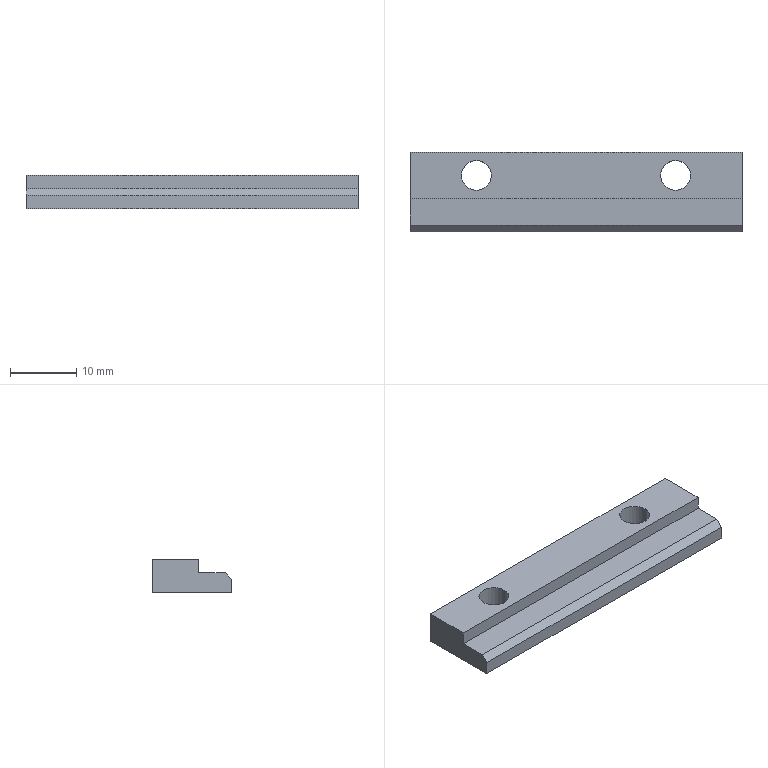Part | SolidWorks | features BaseBody 1 | 1 solid | 13 faces | box 50 x 12 x 5 mm | volume 2316 mm3 | plane 9 | cylinder 4 | commonest cylinder face diameters 4.5 x4
STEP:
#1=CARTESIAN_POINT('',(0.,0.,2.));
#2=VERTEX_POINT('',#1);
#3=CARTESIAN_POINT('',(0.,1.,3.));
#4=VERTEX_POINT('',#3);
#5=CARTESIAN_POINT('',(0.,1.,3.));
#6=DIRECTION('',(0.,0.7071,0.7071));
#7=VECTOR('',#6,1000.);
#8=LINE('',#5,#7);
#9=EDGE_CURVE('',#2,#4,#8,.T.);
#10=ORIENTED_EDGE('',*,*,#9,.F.);
#11=CARTESIAN_POINT('',(50.,0.,2.));
#12=VERTEX_POINT('',#11);
#13=CARTESIAN_POINT('',(0.,0.,2.));
#14=DIRECTION('',(-1.,0.,0.));
#15=VECTOR('',#14,1000.);
#16=LINE('',#13,#15);
#17=EDGE_CURVE('',#12,#2,#16,.T.);
#18=ORIENTED_EDGE('',*,*,#17,.F.);
#19=CARTESIAN_POINT('',(50.,1.,3.));
#20=VERTEX_POINT('',#19);
#21=CARTESIAN_POINT('',(50.,1.,3.));
#22=DIRECTION('',(0.,-0.7071,-0.7071));
#23=VECTOR('',#22,1000.);
#24=LINE('',#21,#23);
#25=EDGE_CURVE('',#20,#12,#24,.T.);
#26=ORIENTED_EDGE('',*,*,#25,.F.);
#27=CARTESIAN_POINT('',(0.,1.,3.));
#28=DIRECTION('',(1.,0.,0.));
#29=VECTOR('',#28,1000.);
#30=LINE('',#27,#29);
#31=EDGE_CURVE('',#4,#20,#30,.T.);
#32=ORIENTED_EDGE('',*,*,#31,.F.);
#33=EDGE_LOOP('',(#10,#18,#26,#32));
#34=FACE_OUTER_BOUND('',#33,.T.);
#35=CARTESIAN_POINT('',(0.,1.,3.));
#36=DIRECTION('',(0.,0.7071,-0.7071));
#37=DIRECTION('',(-1.,0.,0.));
#38=AXIS2_PLACEMENT_3D('',#35,#36,#37);
#39=PLANE('',#38);
#40=ADVANCED_FACE('',(#34),#39,.F.);
#41=CARTESIAN_POINT('',(0.,5.,3.));
#42=VERTEX_POINT('',#41);
#43=CARTESIAN_POINT('',(0.,0.,3.));
#44=DIRECTION('',(0.,1.,0.));
#45=VECTOR('',#44,1000.);
#46=LINE('',#43,#45);
#47=EDGE_CURVE('',#4,#42,#46,.T.);
#48=ORIENTED_EDGE('',*,*,#47,.F.);
#49=ORIENTED_EDGE('',*,*,#31,.T.);
#50=CARTESIAN_POINT('',(50.,5.,3.));
#51=VERTEX_POINT('',#50);
#52=CARTESIAN_POINT('',(50.,0.,3.));
#53=DIRECTION('',(0.,1.,0.));
#54=VECTOR('',#53,1000.);
#55=LINE('',#52,#54);
#56=EDGE_CURVE('',#20,#51,#55,.T.);
#57=ORIENTED_EDGE('',*,*,#56,.T.);
#58=CARTESIAN_POINT('',(0.,5.,3.));
#59=DIRECTION('',(1.,0.,0.));
#60=VECTOR('',#59,1000.);
#61=LINE('',#58,#60);
#62=EDGE_CURVE('',#42,#51,#61,.T.);
#63=ORIENTED_EDGE('',*,*,#62,.F.);
#64=EDGE_LOOP('',(#48,#49,#57,#63));
#65=FACE_OUTER_BOUND('',#64,.T.);
#66=CARTESIAN_POINT('',(0.,0.,3.));
#67=DIRECTION('',(0.,0.,-1.));
#68=DIRECTION('',(0.,-1.,0.));
#69=AXIS2_PLACEMENT_3D('',#66,#67,#68);
#70=PLANE('',#69);
#71=ADVANCED_FACE('',(#65),#70,.F.);
#72=CARTESIAN_POINT('',(50.,5.,5.));
#73=VERTEX_POINT('',#72);
#74=CARTESIAN_POINT('',(50.,5.,5.));
#75=DIRECTION('',(0.,0.,1.));
#76=VECTOR('',#75,1000.);
#77=LINE('',#74,#76);
#78=EDGE_CURVE('',#51,#73,#77,.T.);
#79=ORIENTED_EDGE('',*,*,#78,.T.);
#80=CARTESIAN_POINT('',(0.,5.,5.));
#81=VERTEX_POINT('',#80);
#82=CARTESIAN_POINT('',(0.,5.,5.));
#83=DIRECTION('',(1.,0.,0.));
#84=VECTOR('',#83,1000.);
#85=LINE('',#82,#84);
#86=EDGE_CURVE('',#81,#73,#85,.T.);
#87=ORIENTED_EDGE('',*,*,#86,.F.);
#88=CARTESIAN_POINT('',(0.,5.,5.));
#89=DIRECTION('',(0.,0.,1.));
#90=VECTOR('',#89,1000.);
#91=LINE('',#88,#90);
#92=EDGE_CURVE('',#42,#81,#91,.T.);
#93=ORIENTED_EDGE('',*,*,#92,.F.);
#94=ORIENTED_EDGE('',*,*,#62,.T.);
#95=EDGE_LOOP('',(#79,#87,#93,#94));
#96=FACE_OUTER_BOUND('',#95,.T.);
#97=CARTESIAN_POINT('',(0.,5.,5.));
#98=DIRECTION('',(0.,1.,0.));
#99=DIRECTION('',(1.,0.,0.));
#100=AXIS2_PLACEMENT_3D('',#97,#98,#99);
#101=PLANE('',#100);
#102=ADVANCED_FACE('',(#96),#101,.F.);
#103=CARTESIAN_POINT('',(7.75,8.5,0.));
#104=VERTEX_POINT('',#103);
#105=CARTESIAN_POINT('',(7.75,8.5,5.));
#106=VERTEX_POINT('',#105);
#107=CARTESIAN_POINT('',(7.75,8.5,0.));
#108=DIRECTION('',(0.,0.,1.));
#109=VECTOR('',#108,1000.);
#110=LINE('',#107,#109);
#111=EDGE_CURVE('',#104,#106,#110,.T.);
#112=ORIENTED_EDGE('',*,*,#111,.F.);
#113=CARTESIAN_POINT('',(12.25,8.5,0.));
#114=VERTEX_POINT('',#113);
#115=CARTESIAN_POINT('',(10.,8.5,0.));
#116=DIRECTION('',(0.,0.,1.));
#117=DIRECTION('',(1.,0.,0.));
#118=AXIS2_PLACEMENT_3D('',#115,#116,#117);
#119=CIRCLE('',#118,2.25);
#120=EDGE_CURVE('',#114,#104,#119,.T.);
#121=ORIENTED_EDGE('',*,*,#120,.F.);
#122=CARTESIAN_POINT('',(12.25,8.5,5.));
#123=VERTEX_POINT('',#122);
#124=CARTESIAN_POINT('',(12.25,8.5,0.));
#125=DIRECTION('',(0.,0.,1.));
#126=VECTOR('',#125,1000.);
#127=LINE('',#124,#126);
#128=EDGE_CURVE('',#114,#123,#127,.T.);
#129=ORIENTED_EDGE('',*,*,#128,.T.);
#130=CARTESIAN_POINT('',(10.,8.5,5.));
#131=DIRECTION('',(0.,0.,1.));
#132=DIRECTION('',(1.,0.,0.));
#133=AXIS2_PLACEMENT_3D('',#130,#131,#132);
#134=CIRCLE('',#133,2.25);
#135=EDGE_CURVE('',#123,#106,#134,.T.);
#136=ORIENTED_EDGE('',*,*,#135,.T.);
#137=EDGE_LOOP('',(#112,#121,#129,#136));
#138=FACE_OUTER_BOUND('',#137,.T.);
#139=CARTESIAN_POINT('',(10.,8.5,0.));
#140=DIRECTION('',(0.,0.,1.));
#141=DIRECTION('',(1.,0.,0.));
#142=AXIS2_PLACEMENT_3D('',#139,#140,#141);
#143=CYLINDRICAL_SURFACE('',#142,2.25);
#144=ADVANCED_FACE('',(#138),#143,.F.);
#145=CARTESIAN_POINT('',(37.75,8.5,0.));
#146=VERTEX_POINT('',#145);
#147=CARTESIAN_POINT('',(37.75,8.5,5.));
#148=VERTEX_POINT('',#147);
#149=CARTESIAN_POINT('',(37.75,8.5,0.));
#150=DIRECTION('',(0.,0.,1.));
#151=VECTOR('',#150,1000.);
#152=LINE('',#149,#151);
#153=EDGE_CURVE('',#146,#148,#152,.T.);
#154=ORIENTED_EDGE('',*,*,#153,.F.);
#155=CARTESIAN_POINT('',(42.25,8.5,0.));
#156=VERTEX_POINT('',#155);
#157=CARTESIAN_POINT('',(40.,8.5,0.));
#158=DIRECTION('',(0.,0.,1.));
#159=DIRECTION('',(1.,0.,0.));
#160=AXIS2_PLACEMENT_3D('',#157,#158,#159);
#161=CIRCLE('',#160,2.25);
#162=EDGE_CURVE('',#156,#146,#161,.T.);
#163=ORIENTED_EDGE('',*,*,#162,.F.);
#164=CARTESIAN_POINT('',(42.25,8.5,5.));
#165=VERTEX_POINT('',#164);
#166=CARTESIAN_POINT('',(42.25,8.5,0.));
#167=DIRECTION('',(0.,0.,1.));
#168=VECTOR('',#167,1000.);
#169=LINE('',#166,#168);
#170=EDGE_CURVE('',#156,#165,#169,.T.);
#171=ORIENTED_EDGE('',*,*,#170,.T.);
#172=CARTESIAN_POINT('',(40.,8.5,5.));
#173=DIRECTION('',(0.,0.,1.));
#174=DIRECTION('',(1.,0.,0.));
#175=AXIS2_PLACEMENT_3D('',#172,#173,#174);
#176=CIRCLE('',#175,2.25);
#177=EDGE_CURVE('',#165,#148,#176,.T.);
#178=ORIENTED_EDGE('',*,*,#177,.T.);
#179=EDGE_LOOP('',(#154,#163,#171,#178));
#180=FACE_OUTER_BOUND('',#179,.T.);
#181=CARTESIAN_POINT('',(40.,8.5,0.));
#182=DIRECTION('',(0.,0.,1.));
#183=DIRECTION('',(1.,0.,0.));
#184=AXIS2_PLACEMENT_3D('',#181,#182,#183);
#185=CYLINDRICAL_SURFACE('',#184,2.25);
#186=ADVANCED_FACE('',(#180),#185,.F.);
#187=ORIENTED_EDGE('',*,*,#162,.T.);
#188=CARTESIAN_POINT('',(40.,8.5,0.));
#189=DIRECTION('',(0.,0.,1.));
#190=DIRECTION('',(1.,0.,0.));
#191=AXIS2_PLACEMENT_3D('',#188,#189,#190);
#192=CIRCLE('',#191,2.25);
#193=EDGE_CURVE('',#146,#156,#192,.T.);
#194=ORIENTED_EDGE('',*,*,#193,.T.);
#195=EDGE_LOOP('',(#187,#194));
#196=FACE_BOUND('',#195,.T.);
#197=ORIENTED_EDGE('',*,*,#120,.T.);
#198=CARTESIAN_POINT('',(10.,8.5,0.));
#199=DIRECTION('',(0.,0.,1.));
#200=DIRECTION('',(1.,0.,0.));
#201=AXIS2_PLACEMENT_3D('',#198,#199,#200);
#202=CIRCLE('',#201,2.25);
#203=EDGE_CURVE('',#104,#114,#202,.T.);
#204=ORIENTED_EDGE('',*,*,#203,.T.);
#205=EDGE_LOOP('',(#197,#204));
#206=FACE_BOUND('',#205,.T.);
#207=CARTESIAN_POINT('',(0.,12.,0.));
#208=VERTEX_POINT('',#207);
#209=CARTESIAN_POINT('',(0.,0.,0.));
#210=VERTEX_POINT('',#209);
#211=CARTESIAN_POINT('',(0.,0.,0.));
#212=DIRECTION('',(0.,-1.,0.));
#213=VECTOR('',#212,1000.);
#214=LINE('',#211,#213);
#215=EDGE_CURVE('',#208,#210,#214,.T.);
#216=ORIENTED_EDGE('',*,*,#215,.F.);
#217=CARTESIAN_POINT('',(50.,12.,0.));
#218=VERTEX_POINT('',#217);
#219=CARTESIAN_POINT('',(0.,12.,0.));
#220=DIRECTION('',(-1.,0.,0.));
#221=VECTOR('',#220,1000.);
#222=LINE('',#219,#221);
#223=EDGE_CURVE('',#218,#208,#222,.T.);
#224=ORIENTED_EDGE('',*,*,#223,.F.);
#225=CARTESIAN_POINT('',(50.,0.,0.));
#226=VERTEX_POINT('',#225);
#227=CARTESIAN_POINT('',(50.,0.,0.));
#228=DIRECTION('',(0.,1.,0.));
#229=VECTOR('',#228,1000.);
#230=LINE('',#227,#229);
#231=EDGE_CURVE('',#226,#218,#230,.T.);
#232=ORIENTED_EDGE('',*,*,#231,.F.);
#233=CARTESIAN_POINT('',(0.,0.,0.));
#234=DIRECTION('',(1.,0.,0.));
#235=VECTOR('',#234,1000.);
#236=LINE('',#233,#235);
#237=EDGE_CURVE('',#210,#226,#236,.T.);
#238=ORIENTED_EDGE('',*,*,#237,.F.);
#239=EDGE_LOOP('',(#216,#224,#232,#238));
#240=FACE_OUTER_BOUND('',#239,.T.);
#241=CARTESIAN_POINT('',(0.,0.,0.));
#242=DIRECTION('',(0.,0.,-1.));
#243=DIRECTION('',(0.,-1.,0.));
#244=AXIS2_PLACEMENT_3D('',#241,#242,#243);
#245=PLANE('',#244);
#246=ADVANCED_FACE('',(#196,#206,#240),#245,.T.);
#247=ORIENTED_EDGE('',*,*,#177,.F.);
#248=CARTESIAN_POINT('',(40.,8.5,5.));
#249=DIRECTION('',(0.,0.,1.));
#250=DIRECTION('',(1.,0.,0.));
#251=AXIS2_PLACEMENT_3D('',#248,#249,#250);
#252=CIRCLE('',#251,2.25);
#253=EDGE_CURVE('',#148,#165,#252,.T.);
#254=ORIENTED_EDGE('',*,*,#253,.F.);
#255=EDGE_LOOP('',(#247,#254));
#256=FACE_BOUND('',#255,.T.);
#257=ORIENTED_EDGE('',*,*,#135,.F.);
#258=CARTESIAN_POINT('',(10.,8.5,5.));
#259=DIRECTION('',(0.,0.,1.));
#260=DIRECTION('',(1.,0.,0.));
#261=AXIS2_PLACEMENT_3D('',#258,#259,#260);
#262=CIRCLE('',#261,2.25);
#263=EDGE_CURVE('',#106,#123,#262,.T.);
#264=ORIENTED_EDGE('',*,*,#263,.F.);
#265=EDGE_LOOP('',(#257,#264));
#266=FACE_BOUND('',#265,.T.);
#267=CARTESIAN_POINT('',(0.,12.,5.));
#268=VERTEX_POINT('',#267);
#269=CARTESIAN_POINT('',(0.,0.,5.));
#270=DIRECTION('',(0.,-1.,0.));
#271=VECTOR('',#270,1000.);
#272=LINE('',#269,#271);
#273=EDGE_CURVE('',#268,#81,#272,.T.);
#274=ORIENTED_EDGE('',*,*,#273,.T.);
#275=ORIENTED_EDGE('',*,*,#86,.T.);
#276=CARTESIAN_POINT('',(50.,12.,5.));
#277=VERTEX_POINT('',#276);
#278=CARTESIAN_POINT('',(50.,0.,5.));
#279=DIRECTION('',(0.,1.,0.));
#280=VECTOR('',#279,1000.);
#281=LINE('',#278,#280);
#282=EDGE_CURVE('',#73,#277,#281,.T.);
#283=ORIENTED_EDGE('',*,*,#282,.T.);
#284=CARTESIAN_POINT('',(0.,12.,5.));
#285=DIRECTION('',(-1.,0.,0.));
#286=VECTOR('',#285,1000.);
#287=LINE('',#284,#286);
#288=EDGE_CURVE('',#277,#268,#287,.T.);
#289=ORIENTED_EDGE('',*,*,#288,.T.);
#290=EDGE_LOOP('',(#274,#275,#283,#289));
#291=FACE_OUTER_BOUND('',#290,.T.);
#292=CARTESIAN_POINT('',(0.,0.,5.));
#293=DIRECTION('',(0.,0.,-1.));
#294=DIRECTION('',(0.,-1.,0.));
#295=AXIS2_PLACEMENT_3D('',#292,#293,#294);
#296=PLANE('',#295);
#297=ADVANCED_FACE('',(#256,#266,#291),#296,.F.);
#298=ORIENTED_EDGE('',*,*,#223,.T.);
#299=CARTESIAN_POINT('',(0.,12.,5.));
#300=DIRECTION('',(0.,0.,-1.));
#301=VECTOR('',#300,1000.);
#302=LINE('',#299,#301);
#303=EDGE_CURVE('',#268,#208,#302,.T.);
#304=ORIENTED_EDGE('',*,*,#303,.F.);
#305=ORIENTED_EDGE('',*,*,#288,.F.);
#306=CARTESIAN_POINT('',(50.,12.,5.));
#307=DIRECTION('',(0.,0.,-1.));
#308=VECTOR('',#307,1000.);
#309=LINE('',#306,#308);
#310=EDGE_CURVE('',#277,#218,#309,.T.);
#311=ORIENTED_EDGE('',*,*,#310,.T.);
#312=EDGE_LOOP('',(#298,#304,#305,#311));
#313=FACE_OUTER_BOUND('',#312,.T.);
#314=CARTESIAN_POINT('',(0.,12.,5.));
#315=DIRECTION('',(0.,-1.,0.));
#316=DIRECTION('',(0.,0.,-1.));
#317=AXIS2_PLACEMENT_3D('',#314,#315,#316);
#318=PLANE('',#317);
#319=ADVANCED_FACE('',(#313),#318,.F.);
#320=ORIENTED_EDGE('',*,*,#56,.F.);
#321=ORIENTED_EDGE('',*,*,#25,.T.);
#322=CARTESIAN_POINT('',(50.,0.,5.));
#323=DIRECTION('',(0.,0.,-1.));
#324=VECTOR('',#323,1000.);
#325=LINE('',#322,#324);
#326=EDGE_CURVE('',#12,#226,#325,.T.);
#327=ORIENTED_EDGE('',*,*,#326,.T.);
#328=ORIENTED_EDGE('',*,*,#231,.T.);
#329=ORIENTED_EDGE('',*,*,#310,.F.);
#330=ORIENTED_EDGE('',*,*,#282,.F.);
#331=ORIENTED_EDGE('',*,*,#78,.F.);
#332=EDGE_LOOP('',(#320,#321,#327,#328,#329,#330,#331));
#333=FACE_OUTER_BOUND('',#332,.T.);
#334=CARTESIAN_POINT('',(50.,0.,5.));
#335=DIRECTION('',(-1.,0.,0.));
#336=DIRECTION('',(0.,0.,1.));
#337=AXIS2_PLACEMENT_3D('',#334,#335,#336);
#338=PLANE('',#337);
#339=ADVANCED_FACE('',(#333),#338,.F.);
#340=ORIENTED_EDGE('',*,*,#326,.F.);
#341=ORIENTED_EDGE('',*,*,#17,.T.);
#342=CARTESIAN_POINT('',(0.,0.,5.));
#343=DIRECTION('',(0.,0.,-1.));
#344=VECTOR('',#343,1000.);
#345=LINE('',#342,#344);
#346=EDGE_CURVE('',#2,#210,#345,.T.);
#347=ORIENTED_EDGE('',*,*,#346,.T.);
#348=ORIENTED_EDGE('',*,*,#237,.T.);
#349=EDGE_LOOP('',(#340,#341,#347,#348));
#350=FACE_OUTER_BOUND('',#349,.T.);
#351=CARTESIAN_POINT('',(0.,0.,5.));
#352=DIRECTION('',(0.,1.,0.));
#353=DIRECTION('',(1.,0.,0.));
#354=AXIS2_PLACEMENT_3D('',#351,#352,#353);
#355=PLANE('',#354);
#356=ADVANCED_FACE('',(#350),#355,.F.);
#357=ORIENTED_EDGE('',*,*,#346,.F.);
#358=ORIENTED_EDGE('',*,*,#9,.T.);
#359=ORIENTED_EDGE('',*,*,#47,.T.);
#360=ORIENTED_EDGE('',*,*,#92,.T.);
#361=ORIENTED_EDGE('',*,*,#273,.F.);
#362=ORIENTED_EDGE('',*,*,#303,.T.);
#363=ORIENTED_EDGE('',*,*,#215,.T.);
#364=EDGE_LOOP('',(#357,#358,#359,#360,#361,#362,#363));
#365=FACE_OUTER_BOUND('',#364,.T.);
#366=CARTESIAN_POINT('',(0.,0.,5.));
#367=DIRECTION('',(1.,0.,0.));
#368=DIRECTION('',(0.,1.,0.));
#369=AXIS2_PLACEMENT_3D('',#366,#367,#368);
#370=PLANE('',#369);
#371=ADVANCED_FACE('',(#365),#370,.F.);
#372=ORIENTED_EDGE('',*,*,#193,.F.);
#373=ORIENTED_EDGE('',*,*,#153,.T.);
#374=ORIENTED_EDGE('',*,*,#253,.T.);
#375=ORIENTED_EDGE('',*,*,#170,.F.);
#376=EDGE_LOOP('',(#372,#373,#374,#375));
#377=FACE_OUTER_BOUND('',#376,.T.);
#378=CARTESIAN_POINT('',(40.,8.5,0.));
#379=DIRECTION('',(0.,0.,1.));
#380=DIRECTION('',(1.,0.,0.));
#381=AXIS2_PLACEMENT_3D('',#378,#379,#380);
#382=CYLINDRICAL_SURFACE('',#381,2.25);
#383=ADVANCED_FACE('',(#377),#382,.F.);
#384=ORIENTED_EDGE('',*,*,#203,.F.);
#385=ORIENTED_EDGE('',*,*,#111,.T.);
#386=ORIENTED_EDGE('',*,*,#263,.T.);
#387=ORIENTED_EDGE('',*,*,#128,.F.);
#388=EDGE_LOOP('',(#384,#385,#386,#387));
#389=FACE_OUTER_BOUND('',#388,.T.);
#390=CARTESIAN_POINT('',(10.,8.5,0.));
#391=DIRECTION('',(0.,0.,1.));
#392=DIRECTION('',(1.,0.,0.));
#393=AXIS2_PLACEMENT_3D('',#390,#391,#392);
#394=CYLINDRICAL_SURFACE('',#393,2.25);
#395=ADVANCED_FACE('',(#389),#394,.F.);
#396=CLOSED_SHELL('',(#40,#71,#102,#144,#186,#246,#297,#319,#339,#356,#371,#383,#395));
#397=MANIFOLD_SOLID_BREP('',#396);
#398=CARTESIAN_POINT('',(0.,0.,0.));
#399=DIRECTION('',(0.,0.,1.));
#400=DIRECTION('',(1.,0.,0.));
#401=AXIS2_PLACEMENT_3D('',#398,#399,#400);
#402=(LENGTH_UNIT()NAMED_UNIT(*)SI_UNIT(.MILLI.,.METRE.));
#403=UNCERTAINTY_MEASURE_WITH_UNIT(LENGTH_MEASURE(0.00001),#402,'','');
#404=(NAMED_UNIT(*)PLANE_ANGLE_UNIT()SI_UNIT($,.RADIAN.));
#405=(NAMED_UNIT(*)SI_UNIT($,.STERADIAN.)SOLID_ANGLE_UNIT());
#406=(GEOMETRIC_REPRESENTATION_CONTEXT(3)GLOBAL_UNCERTAINTY_ASSIGNED_CONTEXT((#403))GLOBAL_UNIT_ASSIGNED_CONTEXT((#402,#404,#405))REPRESENTATION_CONTEXT('',''));
#407=ADVANCED_BREP_SHAPE_REPRESENTATION('',(#397,#401),#406);